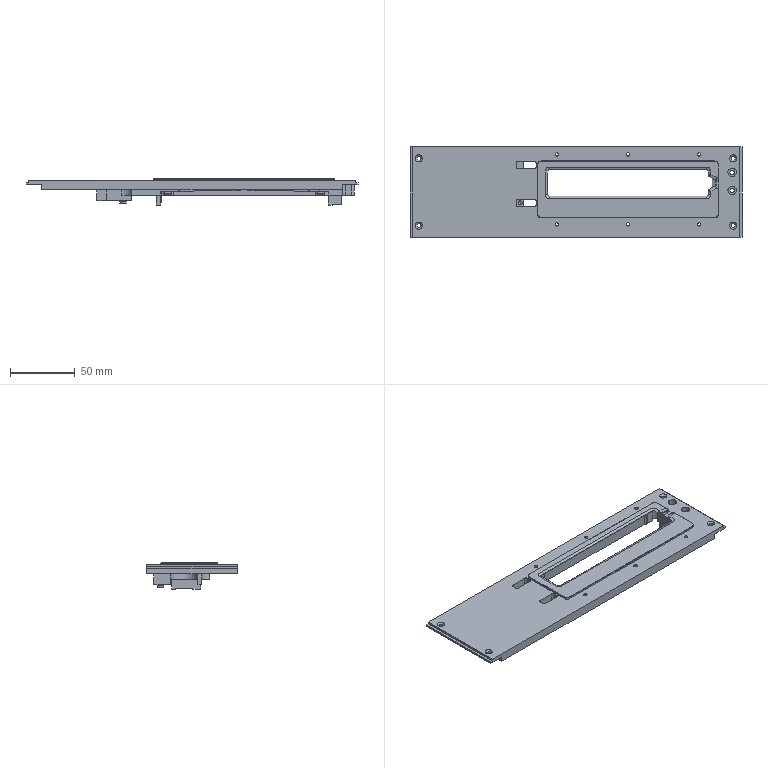NC program | NX | posted with a generic post | part box 256.6 x 70.3 x 20.422 mm
Lines 61 to 1223 of 23702:
(CAVITY_MILL , TOOL : D10)
N120 T10 M6
N122 G54
N124 G17 G0 G90 X-34.437 Y-41.146 S9500 M3
N126 G43 Z30. H10
N128 Z0.863
N130 G94 G1 Z-0.637 F1000.
N132 X-37.323 Y-36.146
N134 G3 X-38.189 Y-35.646 R1.
N136 G1 X-128.303 F3000.
N138 G2 X-128.797 Y-35.152 R0.494
N140 G1 Y35.152
N142 G2 X-128.303 Y35.646 R0.494
N144 G1 X128.303
N146 G2 X128.797 Y35.152 R0.494
N148 G1 Y-35.152
N150 G2 X128.303 Y-35.646 R0.494
N152 G1 X-38.189
N154 Y-29.646
N156 X-122.797
N158 Y29.646
N160 X122.797
N162 Y-29.646
N164 X-38.189
N166 Y-23.646
N168 X-116.797
N170 Y23.646
N172 X116.797
N174 Y-23.646
N176 X-38.189
N178 Y-17.646
N180 X-110.797
N182 Y-12.457
N184 G3 X-108.238 Y-13. R6.3
N186 G1 X-105.19
N188 G3 X-98.89 Y-6.7 R6.3
N190 G1 Y-0.604
N192 G3 X-105.19 Y5.696 R6.3
N194 G1 X-108.238
N196 G3 X-110.797 Y5.153 R6.3
N198 G1 X-110.31 Y4.056
N200 G2 X-108.238 Y4.496 R5.1
N202 G1 X-105.19
N204 G2 X-100.09 Y-0.604 R5.1
N206 G1 Y-6.7
N208 G2 X-105.19 Y-11.8 R5.1
N210 G1 X-108.238
N212 G2 X-113.338 Y-6.7 R5.1
N214 G1 Y-0.604
N216 G2 X-110.31 Y4.056 R5.1
N218 G1 X-110.797 Y5.153
N220 Y17.646
N222 X18.206
N224 G3 X17.898 Y15.7 R6.3
N226 G1 Y12.604
N228 G3 X24.198 Y6.304 R6.3
N230 G1 X27.754
N232 G3 X34.054 Y12.604 R6.3
N234 G1 Y15.7
N236 G3 X33.746 Y17.646 R6.3
N238 G1 X32.604 Y17.276
N240 G2 X32.854 Y15.7 R5.1
N242 G1 Y12.604
N244 G2 X27.754 Y7.504 R5.1
N246 G1 X24.198
N248 G2 X19.098 Y12.604 R5.1
N250 G1 Y15.7
N252 G2 X24.198 Y20.8 R5.1
N254 G1 X27.754
N256 G2 X32.604 Y17.276 R5.1
N258 G1 X33.746 Y17.646
N260 X110.797
N262 Y-17.646
N264 X31.656
N266 Y-11.646
N268 G3 X34.054 Y-6.7 R6.3
N270 G1 Y-0.604
N272 G3 X33.587 Y1.775 R6.3
N274 X40.016 Y11.646 R12.3
N276 G1 X104.797
N278 Y-11.646
N280 X31.656
N282 X40.054 Y-5.646
N284 Y-0.946
N286 G3 X44.68 Y5.646 R18.3
N288 G1 X98.797
N290 Y-5.646
N292 X40.054
N294 X45.941 Y-1.146
N296 G3 X47.466 Y1.146 R22.8
N298 G1 X94.297
N300 Y-1.146
N302 X45.941
N304 X40.054 Y-5.646
N306 X31.656 Y-11.646
N308 Y-17.646
N310 X-38.189
N312 Y-11.646
N314 X-93.928
N316 G3 X-92.89 Y-6.7 R12.3
N318 G1 Y-0.604
N320 G3 X-104.086 Y11.646 R12.3
N322 G1 X11.935
N324 G3 X18.364 Y1.775 R12.3
N326 X17.898 Y-0.604 R6.3
N328 G1 Y-6.7
N330 G3 X20.296 Y-11.646 R6.3
N332 G1 X21.039 Y-10.704
N334 G2 X19.098 Y-6.7 R5.1
N336 G1 Y-0.604
N338 G2 X24.198 Y4.496 R5.1
N340 G1 X27.754
N342 G2 X32.854 Y-0.604 R5.1
N344 G1 Y-6.7
N346 G2 X27.754 Y-11.8 R5.1
N348 G1 X24.198
N350 G2 X21.039 Y-10.704 R5.1
N352 G1 X20.296 Y-11.646
N354 X-38.189
N356 Y-5.646
N358 X-86.89
N360 Y-0.604
N362 G3 X-87.99 Y5.646 R18.3
N364 G1 X7.272
N366 G3 X11.898 Y-0.946 R18.3
N368 G1 Y-5.646
N370 X-38.189
N372 Y-1.146
N374 X-82.39
N376 Y-0.604
N378 G3 X-82.457 Y1.146 R22.8
N380 G1 X4.486
N382 G3 X6.011 Y-1.146 R22.8
N384 G1 X-38.189
N386 G3 X-39.056 Y-1.646 R1.
N388 G1 Z0.863
N390 G0 Z30.
N392 X-33.743 Y-41.146
N394 Z0.482
N396 G1 Z-1.018 F1000.
N398 X-36.63 Y-36.146
N400 G3 X-37.496 Y-35.646 R1.
N402 G1 X-128.303 F3000.
N404 G2 X-128.797 Y-35.152 R0.494
N406 G1 Y35.152
N408 G2 X-128.303 Y35.646 R0.494
N410 G1 X128.303
N412 G2 X128.797 Y35.152 R0.494
N414 G1 Y-35.152
N416 G2 X128.303 Y-35.646 R0.494
N418 G1 X-37.496
N420 Y-29.646
N422 X-122.797
N424 Y29.646
N426 X122.797
N428 Y-29.646
N430 X-37.496
N432 Y-23.646
N434 X-116.797
N436 Y-12.864
N438 G3 X-115.496 Y-13. R6.3
N440 G1 X-105.19
N442 G3 X-98.89 Y-6.7 R6.3
N444 G1 Y14.085
N446 G3 X-105.19 Y20.385 R6.3
N448 G1 X-115.496
N450 G3 X-116.797 Y20.249 R6.3
N452 G1 X-116.549 Y19.075
N454 G2 X-115.496 Y19.185 R5.1
N456 G1 X-105.19
N458 G2 X-100.09 Y14.085 R5.1
N460 G1 Y-6.7
N462 G2 X-105.19 Y-11.8 R5.1
N464 G1 X-115.496
N466 G2 X-120.596 Y-6.7 R5.1
N468 G1 Y14.085
N470 G2 X-116.549 Y19.075 R5.1
N472 G1 X-116.797 Y20.249
N474 Y23.646
N476 X116.797
N478 Y-23.646
N480 X-37.496
N482 Y-17.646
N484 X-99.58
N486 X-108.161 Y-18.324
N488 X-99.58 Y-17.646
N490 G3 X-92.89 Y-6.7 R12.3
N492 G1 Y14.085
N494 G3 X-93.417 Y17.646 R12.3
N496 G1 X18.206
N498 G3 X17.898 Y15.7 R6.3
N500 G1 Y12.604
N502 G3 X18.677 Y9.57 R6.3
N504 G1 Y2.43
N506 G3 X17.898 Y-0.604 R6.3
N508 G1 Y-6.7
N510 G3 X24.198 Y-13. R6.3
N512 G1 X27.754
N514 G3 X34.054 Y-6.7 R6.3
N516 G1 Y15.7
N518 G3 X33.746 Y17.646 R6.3
N520 G1 X32.604 Y17.276
N522 G2 X32.854 Y15.7 R5.1
N524 G1 Y-6.7
N526 G2 X27.754 Y-11.8 R5.1
N528 G1 X24.198
N530 G2 X19.098 Y-6.7 R5.1
N532 G1 Y-0.604
N534 G2 X19.877 Y2.105 R5.1
N536 G1 Y9.895
N538 G2 X19.098 Y12.604 R5.1
N540 G1 Y15.7
N542 G2 X24.198 Y20.8 R5.1
N544 G1 X27.754
N546 G2 X32.604 Y17.276 R5.1
N548 G1 X33.746 Y17.646
N550 X110.797
N552 Y-17.646
N554 X39.015
N556 Y-11.646
N558 G3 X40.054 Y-6.7 R12.3
N560 G1 Y11.646
N562 X104.797
N564 Y-11.646
N566 X39.015
N568 X46.054 Y-5.646
N570 Y5.646
N572 X98.797
N574 Y-5.646
N576 X46.054
N578 X50.554 Y-1.146
N580 Y1.146
N582 X94.297
N584 Y-1.146
N586 X50.554
N588 X46.054 Y-5.646
N590 X39.015 Y-11.646
N592 Y-17.646
N594 X-37.496
N596 Y-11.646
N598 X-87.571
N600 G3 X-86.89 Y-6.7 R18.3
N602 G1 Y11.646
N604 X11.935
N606 G3 X12.677 Y8.297 R12.3
N608 G1 Y3.703
N610 G3 X11.898 Y-0.604 R12.3
N612 G1 Y-6.7
N614 G3 X12.936 Y-11.646 R12.3
N616 G1 X-37.496
N618 Y-5.646
N620 X-80.89
N622 Y5.646
N624 X6.677
N626 Y4.677
N628 G3 X5.898 Y-0.604 R18.3
N630 G1 Y-5.646
N632 X-37.496
N634 Y-1.146
N636 X-76.39
N638 Y1.146
N640 X1.465
N642 G3 X1.398 Y-0.604 R22.8
N644 G1 Y-1.146
N646 X-37.496
N648 G3 X-38.362 Y-1.646 R1.
N650 G1 Z0.482
N652 G0 Z30.
N654 X-33.743 Y-41.146
N656 Z0.078
N658 G1 Z-1.422 F1000.
N660 X-36.63 Y-36.146
N662 G3 X-37.496 Y-35.646 R1.
N664 G1 X-128.303 F3000.
N666 G2 X-128.797 Y-35.152 R0.495
N668 G1 Y35.152
N670 G2 X-128.303 Y35.646 R0.495
N672 G1 X128.303
N674 G2 X128.797 Y35.152 R0.495
N676 G1 Y-35.152
N678 G2 X128.303 Y-35.646 R0.495
N680 G1 X-37.496
N682 Y-29.646
N684 X-122.797
N686 Y29.646
N688 X122.797
N690 Y-29.646
N692 X-37.496
N694 Y-23.646
N696 X-116.797
N698 Y-12.864
N700 G3 X-115.496 Y-13. R6.3
N702 G1 X-105.19
N704 G3 X-98.89 Y-6.7 R6.3
N706 G1 Y14.085
N708 G3 X-105.19 Y20.385 R6.3
N710 G1 X-115.496
N712 G3 X-116.797 Y20.249 R6.3
N714 G1 X-116.549 Y19.075
N716 G2 X-115.496 Y19.185 R5.1
N718 G1 X-105.19
N720 G2 X-100.09 Y14.085 R5.1
N722 G1 Y-6.7
N724 G2 X-105.19 Y-11.8 R5.1
N726 G1 X-115.496
N728 G2 X-120.596 Y-6.7 R5.1
N730 G1 Y14.085
N732 G2 X-116.549 Y19.075 R5.1
N734 G1 X-116.797 Y20.249
N736 Y23.646
N738 X116.797
N740 Y-23.646
N742 X-37.496
N744 Y-17.646
N746 X-99.58
N748 X-108.161 Y-18.324
N750 X-99.58 Y-17.646
N752 G3 X-92.89 Y-6.7 R12.3
N754 G1 Y14.085
N756 G3 X-93.417 Y17.646 R12.3
N758 G1 X18.206
N760 G3 X17.898 Y15.7 R6.3
N762 G1 Y12.604
N764 G3 X18.273 Y10.464 R6.3
N766 G1 Y1.536
N768 G3 X17.898 Y-0.604 R6.3
N770 G1 Y-6.7
N772 G3 X24.198 Y-13. R6.3
N774 G1 X27.754
N776 G3 X34.054 Y-6.7 R6.3
N778 G1 Y15.7
N780 G3 X33.746 Y17.646 R6.3
N782 G1 X32.604 Y17.276
N784 G2 X32.854 Y15.7 R5.1
N786 G1 Y-6.7
N788 G2 X27.754 Y-11.8 R5.1
N790 G1 X24.198
N792 G2 X19.098 Y-6.7 R5.1
N794 G1 Y-0.604
N796 G2 X19.473 Y1.315 R5.1
N798 G1 Y10.685
N800 G2 X19.098 Y12.604 R5.1
N802 G1 Y15.7
N804 G2 X24.198 Y20.8 R5.1
N806 G1 X27.754
N808 G2 X32.604 Y17.276 R5.1
N810 G1 X33.746 Y17.646
N812 X110.797
N814 Y-17.646
N816 X39.015
N818 Y-11.646
N820 G3 X40.054 Y-6.7 R12.3
N822 G1 Y11.646
N824 X104.797
N826 Y-11.646
N828 X39.015
N830 X46.054 Y-5.646
N832 Y5.646
N834 X98.797
N836 Y-5.646
N838 X46.054
N840 X50.554 Y-1.146
N842 Y1.146
N844 X94.297
N846 Y-1.146
N848 X50.554
N850 X46.054 Y-5.646
N852 X39.015 Y-11.646
N854 Y-17.646
N856 X-37.496
N858 Y-11.646
N860 X-87.571
N862 G3 X-86.89 Y-6.7 R18.3
N864 G1 Y11.646
N866 X11.935
N868 G3 X12.273 Y9.591 R12.3
N870 G1 Y2.409
N872 G3 X11.898 Y-0.604 R12.3
N874 G1 Y-6.7
N876 G3 X12.936 Y-11.646 R12.3
N878 G1 X-37.496
N880 Y-5.646
N882 X-80.89
N884 Y5.646
N886 X6.273
N888 Y3.08
N890 G3 X5.898 Y-0.604 R18.3
N892 G1 Y-5.646
N894 X-37.496
N896 Y-1.146
N898 X-76.39
N900 Y1.146
N902 X1.465
N904 G3 X1.398 Y-0.604 R22.8
N906 G1 Y-1.146
N908 X-37.496
N910 G3 X-38.362 Y-1.646 R1.
N912 G1 Z0.078
N914 G0 X-33.743 Y-41.147 Z-0.922
N916 G1 Z-2.422 F1000.
N918 X-36.63 Y-36.147
N920 G3 X-37.496 Y-35.647 R1.
N922 G1 X-128.302 F3000.
N924 G2 X-128.797 Y-35.152 R0.495
N926 G1 Y35.152
N928 G2 X-128.302 Y35.647 R0.495
N930 G1 X128.302
N932 G2 X128.797 Y35.152 R0.495
N934 G1 Y-35.152
N936 G2 X128.302 Y-35.647 R0.495
N938 G1 X-37.496
N940 Y-29.647
N942 X-122.797
N944 Y29.647
N946 X46.173
N948 G3 X60.355 Y29.647 R-8.792
N950 G1 X59.387 Y28.937
N952 G2 X57.751 Y18.327 R7.592
N954 X59.387 Y28.937 R-7.592
N956 G1 X60.355 Y29.647
N958 X122.797
N960 Y-29.647
N962 X-37.496
N964 Y-23.647
N966 X-116.797
N968 Y-12.864
N970 G3 X-115.496 Y-13. R6.3
N972 G1 X-105.19
N974 G3 X-98.89 Y-6.7 R6.3
N976 G1 Y14.085
N978 G3 X-105.19 Y20.385 R6.3
N980 G1 X-115.496
N982 G3 X-116.797 Y20.249 R6.3
N984 G1 X-116.549 Y19.075
N986 G2 X-115.496 Y19.185 R5.1
N988 G1 X-105.19
N990 G2 X-100.09 Y14.085 R5.1
N992 G1 Y-6.7
N994 G2 X-105.19 Y-11.8 R5.1
N996 G1 X-115.496
N998 G2 X-120.596 Y-6.7 R5.1
N1000 G1 Y14.085
N1002 G2 X-116.549 Y19.075 R5.1
N1004 G1 X-116.797 Y20.249
N1006 Y23.647
N1008 X38.494
N1010 G3 X68.034 Y23.647 R14.792
N1012 G1 X116.797
N1014 Y-23.647
N1016 X-37.496
N1018 Y-17.647
N1020 X-99.581
N1022 X-108.162 Y-18.324
N1024 X-99.581 Y-17.647
N1026 G3 X-92.89 Y-6.7 R12.3
N1028 G1 Y14.085
N1030 G3 X-93.417 Y17.647 R12.3
N1032 G1 X18.206
N1034 G3 X17.898 Y15.7 R6.3
N1036 G1 Y10.868
N1038 G3 X17.491 Y8.642 R6.3
N1040 G1 Y3.358
N1042 G3 X17.898 Y1.132 R6.3
N1044 G1 Y-6.7
N1046 G3 X24.198 Y-13. R6.3
N1048 G1 X27.754
N1050 G3 X34.054 Y-6.7 R6.3
N1052 G1 Y15.7
N1054 G3 X33.976 Y16.687 R6.3
N1056 G1 X32.791 Y16.499
N1058 G2 X32.854 Y15.7 R5.1
N1060 G1 Y-6.7
N1062 G2 X27.754 Y-11.8 R5.1
N1064 G1 X24.198
N1066 G2 X19.098 Y-6.7 R5.1
N1068 G1 Y1.363
N1070 G2 X18.691 Y3.358 R5.1
N1072 G1 Y8.642
N1074 G2 X19.098 Y10.637 R5.1
N1076 G1 Y15.7
N1078 G2 X24.198 Y20.8 R5.1
N1080 G1 X27.754
N1082 G2 X32.791 Y16.499 R5.1
N1084 G1 X33.976 Y16.687
N1086 G3 X72.911 Y17.647 R20.792
N1088 G1 X110.797
N1090 Y-17.647
N1092 X39.015
N1094 Y-11.647
N1096 G3 X40.054 Y-6.647 R12.3
N1098 G1 X45.576 Y-6.521
N1100 X40.054 Y-6.647
N1102 Y1.142
N1104 G3 X76.798 Y11.647 R26.792
N1106 G1 X104.797
N1108 Y-11.647
N1110 X66.283
N1112 Y-5.647
N1114 G3 X80.129 Y5.647 R32.792
N1116 G1 X98.797
N1118 Y-5.647
N1120 X80.384
N1122 Y-1.147
N1124 G3 X82.378 Y1.147 R37.292
N1126 G1 X94.297
N1128 Y-1.147
N1130 X80.384
N1132 Y-5.647
N1134 X66.283
N1136 X60.869 Y-6.534
N1138 X66.283 Y-5.647
N1140 Y-11.647
N1142 X39.015
N1144 Y-17.647
N1146 X-37.496
N1148 Y-11.647
N1150 X-87.571
N1152 G3 X-86.89 Y-6.7 R18.3
N1154 G1 Y11.647
N1156 X11.864
N1158 G3 X11.491 Y8.642 R12.3
N1160 G1 Y3.358
N1162 G3 X11.898 Y0.223 R12.3
N1164 G1 Y-6.7
N1166 G3 X12.936 Y-11.647 R12.3
N1168 G1 X-37.496
N1170 Y-5.647
N1172 X-80.89
N1174 Y5.647
N1176 X5.491
N1178 Y3.358
N1180 G3 X5.898 Y-0.477 R18.3
N1182 G1 Y-5.647
N1184 X-37.496
N1186 Y-1.147
N1188 X-76.39
N1190 Y1.147
N1192 X1.099
N1194 G3 X1.398 Y-0.927 R22.8
N1196 G1 Y-1.147
N1198 X-37.496
N1200 G3 X-38.362 Y-1.647 R1.
N1202 G1 Z-0.922
N1204 G0 X-33.743 Y-41.147 Z-1.922
N1206 G1 Z-3.422 F1000.
N1208 X-36.63 Y-36.147
N1210 G3 X-37.496 Y-35.647 R1.
N1212 G1 X-128.302 F3000.
N1214 G2 X-128.797 Y-35.152 R0.495
N1216 G1 Y35.152
N1218 G2 X-128.302 Y35.647 R0.495
N1220 G1 X128.302
N1222 G2 X128.797 Y35.152 R0.495
N1224 G1 Y-35.152
N1226 G2 X128.302 Y-35.647 R0.495
N1228 G1 X-37.496
N1230 Y-29.647
N1232 X-122.797
N1234 Y29.647
N1236 X46.162
N1238 G3 X60.366 Y29.647 R-8.8
N1240 G1 X59.397 Y28.938
N1242 G2 X57.752 Y18.317 R7.6
N1244 X59.397 Y28.938 R-7.6
N1246 G1 X60.366 Y29.647
N1248 X122.797
N1250 Y-29.647
N1252 X-37.496
N1254 Y-23.647
N1256 X-116.797
N1258 Y-12.864
N1260 G3 X-115.496 Y-13. R6.3
N1262 G1 X-105.19
N1264 G3 X-98.89 Y-6.7 R6.3
N1266 G1 Y14.085
N1268 G3 X-105.19 Y20.385 R6.3
N1270 G1 X-115.496
N1272 G3 X-116.797 Y20.249 R6.3
N1274 G1 X-116.55 Y19.075
N1276 G2 X-115.496 Y19.185 R5.1
N1278 G1 X-105.19
N1280 G2 X-100.09 Y14.085 R5.1
N1282 G1 Y-6.7
N1284 G2 X-105.19 Y-11.8 R5.1
N1286 G1 X-115.496
N1288 G2 X-120.596 Y-6.7 R5.1
N1290 G1 Y14.085
N1292 G2 X-116.55 Y19.075 R5.1
N1294 G1 X-116.797 Y20.249
N1296 Y23.647
N1298 X38.486
N1300 G3 X68.042 Y23.647 R14.8
N1302 G1 X116.797
N1304 Y-23.647
N1306 X-37.496
N1308 Y-17.647
N1310 X-99.581
N1312 X-108.162 Y-18.324
N1314 X-99.581 Y-17.647
N1316 G3 X-92.89 Y-6.7 R12.3
N1318 G1 Y14.085
N1320 G3 X-93.417 Y17.647 R12.3
N1322 G1 X18.206
N1324 G3 X17.898 Y15.7 R6.3
N1326 G1 Y10.868
N1328 G3 X17.491 Y8.642 R6.3
N1330 G1 Y3.358
N1332 G3 X17.898 Y1.132 R6.3
N1334 G1 Y-6.7
N1336 G3 X24.198 Y-13. R6.3
N1338 G1 X27.754
N1340 G3 X34.054 Y-6.7 R6.3
N1342 G1 Y15.7
N1344 G3 X33.982 Y16.65 R6.3
N1346 G1 X32.795 Y16.469
N1348 G2 X32.854 Y15.7 R5.1
N1350 G1 Y-6.7
N1352 G2 X27.754 Y-11.8 R5.1
N1354 G1 X24.198
N1356 G2 X19.098 Y-6.7 R5.1
N1358 G1 Y1.363
N1360 G2 X18.691 Y3.358 R5.1
N1362 G1 Y8.642
N1364 G2 X19.098 Y10.637 R5.1
N1366 G1 Y15.7
N1368 G2 X24.198 Y20.8 R5.1
N1370 G1 X27.754
N1372 G2 X32.795 Y16.469 R5.1
N1374 G1 X33.982 Y16.65
N1376 G3 X72.92 Y17.647 R20.8
N1378 G1 X110.797
N1380 Y-17.647
N1382 X39.015
N1384 Y-11.647
N1386 G3 X40.054 Y-6.647 R12.3
N1388 G1 X45.564 Y-6.524
N1390 X40.054 Y-6.647
N1392 Y1.132
N1394 G3 X76.808 Y11.647 R26.8
N1396 G1 X104.797
N1398 Y-11.647
N1400 X66.303
N1402 Y-5.647
N1404 G3 X80.139 Y5.647 R32.8
N1406 G1 X98.797
N1408 Y-5.647
N1410 X80.395
N1412 Y-1.147
N1414 G3 X82.389 Y1.147 R37.3
N1416 G1 X94.297
N1418 Y-1.147
N1420 X80.395
N1422 Y-5.647
N1424 X66.303
N1426 X60.896 Y-6.535
N1428 X66.303 Y-5.647
N1430 Y-11.647
N1432 X39.015
N1434 Y-17.647
N1436 X-37.496
N1438 Y-11.647
N1440 X-87.571
N1442 G3 X-86.89 Y-6.7 R18.3
N1444 G1 Y11.647
N1446 X11.864
N1448 G3 X11.491 Y8.642 R12.3
N1450 G1 Y3.358
N1452 G3 X11.898 Y0.223 R12.3
N1454 G1 Y-6.7
N1456 G3 X12.936 Y-11.647 R12.3
N1458 G1 X-37.496
N1460 Y-5.647
N1462 X-80.89
N1464 Y5.647
N1466 X5.491
N1468 Y3.358
N1470 G3 X5.898 Y-0.477 R18.3
N1472 G1 Y-5.647
N1474 X-37.496
N1476 Y-1.147
N1478 X-76.39
N1480 Y1.147
N1482 X1.099
N1484 G3 X1.398 Y-0.927 R22.8
N1486 G1 Y-1.147
N1488 X-37.496
N1490 G3 X-38.362 Y-1.647 R1.
N1492 G1 Z-1.922
N1494 G0 X-33.743 Y-41.147 Z-2.762
N1496 G1 Z-4.262 F1000.
N1498 X-36.63 Y-36.147
N1500 G3 X-37.496 Y-35.647 R1.
N1502 G1 X-128.302 F3000.
N1504 G2 X-128.798 Y-35.152 R0.495
N1506 G1 Y35.152
N1508 G2 X-128.302 Y35.647 R0.495
N1510 G1 X45.124
N1512 G2 X46.504 Y35.8 R6.3
N1514 G1 X73.504
N1516 G2 X74.884 Y35.647 R6.3
N1518 G1 X128.302
N1520 G2 X128.798 Y35.152 R0.495
N1522 G1 Y-35.152
N1524 G2 X128.302 Y-35.647 R0.495
N1526 G1 X-37.496
N1528 Y-29.647
N1530 X-122.798
N1532 Y29.647
N1534 X40.206
N1536 X40.204 Y29.5
N1538 Y17.029
N1540 Y16.501
N1542 G3 X46.504 Y10.2 R6.301
N1544 G1 X73.504
N1546 G3 X79.804 Y16.5 R6.3
N1548 G1 Y29.5
N1550 X79.802 Y29.647
N1552 X78.603 Y29.619
N1554 X78.604 Y29.5
N1556 Y16.5
N1558 G2 X73.504 Y11.4 R5.1
N1560 G1 X46.504
N1562 G2 X41.404 Y16.5 R5.101
N1564 G1 Y17.029
N1566 Y29.5
N1568 G2 X46.504 Y34.6 R5.1
N1570 G1 X73.504
N1572 G2 X78.603 Y29.619 R5.1
N1574 G1 X79.802 Y29.647
N1576 X122.798
N1578 Y-29.647
N1580 X-37.496
N1582 Y-23.647
N1584 X-116.798
N1586 Y-12.864
N1588 G3 X-115.496 Y-13. R6.3
N1590 G1 X-105.19
N1592 G3 X-98.89 Y-6.7 R6.3
N1594 G1 Y14.085
N1596 G3 X-105.19 Y20.385 R6.3
N1598 G1 X-115.496
N1600 G3 X-116.798 Y20.249 R6.3
N1602 G1 X-116.55 Y19.075
N1604 G2 X-115.496 Y19.185 R5.1
N1606 G1 X-105.19
N1608 G2 X-100.09 Y14.085 R5.1
N1610 G1 Y-6.7
N1612 G2 X-105.19 Y-11.8 R5.1
N1614 G1 X-115.496
N1616 G2 X-120.596 Y-6.7 R5.1
N1618 G1 Y14.085
N1620 G2 X-116.55 Y19.075 R5.1
N1622 G1 X-116.798 Y20.249
N1624 Y23.647
N1626 X34.204
N1628 Y17.031
N1630 Y16.5
N1632 G3 X46.502 Y4.2 R12.301
N1634 G1 X73.504
N1636 G3 X85.804 Y16.5 R12.3
N1638 G1 Y23.647
N1640 X116.798
N1642 Y-23.647
N1644 X-37.496
N1646 Y-17.647
N1648 X-99.581
N1650 X-108.162 Y-18.324
N1652 X-99.581 Y-17.647
N1654 G3 X-92.89 Y-6.7 R12.3
N1656 G1 Y14.085
N1658 G3 X-93.417 Y17.647 R12.3
N1660 G1 X18.206
N1662 G3 X17.898 Y15.7 R6.3
N1664 G1 Y10.868
N1666 G3 X17.491 Y8.642 R6.3
N1668 G1 Y3.358
N1670 G3 X17.898 Y1.132 R6.3
N1672 G1 Y-6.7
N1674 G3 X24.198 Y-13. R6.3
N1676 G1 X27.754
N1678 G3 X34.054 Y-6.7 R6.3
N1680 G1 Y3.088
N1682 X32.854
N1684 Y-6.7
N1686 G2 X27.754 Y-11.8 R5.1
N1688 G1 X24.198
N1690 G2 X19.098 Y-6.7 R5.1
N1692 G1 Y1.363
N1694 G2 X18.691 Y3.358 R5.1
N1696 G1 Y8.642
N1698 G2 X19.098 Y10.637 R5.1
N1700 G1 Y15.7
N1702 G2 X24.198 Y20.8 R5.1
N1704 G1 X27.754
N1706 G2 X32.854 Y15.7 R5.1
N1708 G1 Y3.088
N1710 X34.054
N1712 G3 X41.247 Y-1.028 R18.301
N1714 X40.204 Y-4.5 R6.3
N1716 G1 Y-7.5
N1718 G3 X46.504 Y-13.8 R6.3
N1720 G1 X66.004
N1722 G3 X72.304 Y-7.5 R6.3
N1724 G1 Y-4.5
N1726 G3 X71.696 Y-1.8 R6.3
N1728 G1 X70.612 Y-2.314
N1730 G2 X71.104 Y-4.5 R5.1
N1732 G1 Y-7.5
N1734 G2 X66.004 Y-12.6 R5.1
N1736 G1 X46.504
N1738 G2 X41.404 Y-7.5 R5.1
N1740 G1 Y-4.5
N1742 G2 X46.504 Y0.6 R5.1
N1744 G1 X66.004
N1746 G2 X70.612 Y-2.314 R5.1
N1748 G1 X71.696 Y-1.8
N1750 X73.504
N1752 G3 X91.804 Y16.5 R18.3
N1754 G1 Y17.647
N1756 X110.798
N1758 Y-17.647
N1760 X77.584
N1762 Y-11.647
N1764 G3 X78.304 Y-7.5 R12.3
N1766 G1 Y-7.321
N1768 G3 X97.314 Y11.647 R24.3
N1770 G1 X104.798
N1772 Y-11.647
N1774 X94.183
N1776 Y-5.647
N1778 G3 X98.798 Y-0.183 R30.3
N1780 G1 Y-5.647
N1782 X94.183
N1784 Y-11.647
N1786 X77.584
N1788 Y-17.647
N1790 X-37.496
N1792 Y-11.647
N1794 X-87.571
N1796 G3 X-86.89 Y-6.7 R18.3
N1798 G1 Y11.647
N1800 X11.864
N1802 G3 X11.491 Y8.642 R12.3
N1804 G1 Y3.358
N1806 G3 X11.898 Y0.223 R12.3
N1808 G1 Y-6.7
N1810 G3 X12.937 Y-11.647 R12.3
N1812 G1 X-37.496
N1814 Y-5.647
N1816 X-80.89
N1818 Y5.647
N1820 X5.491
N1822 Y3.358
N1824 G3 X5.898 Y-0.477 R18.3
N1826 G1 Y-5.647
N1828 X-37.496
N1830 Y-1.147
N1832 X-76.39
N1834 Y1.147
N1836 X1.099
N1838 G3 X1.398 Y-0.927 R22.8
N1840 G1 Y-1.147
N1842 X-37.496
N1844 G3 X-38.362 Y-1.647 R1.
N1846 G1 Z-2.762
N1848 G0 X-33.743 Y-41.147 Z-3.602
N1850 G1 Z-5.102 F1000.
N1852 X-36.63 Y-36.147
N1854 G3 X-37.496 Y-35.647 R1.
N1856 G1 X-128.302 F3000.
N1858 G2 X-128.798 Y-35.152 R0.496
N1860 G1 Y35.152
N1862 G2 X-128.302 Y35.647 R0.496
N1864 G1 X45.125
N1866 G2 X46.504 Y35.8 R6.3
N1868 G1 X73.504
N1870 G2 X74.883 Y35.647 R6.3
N1872 G1 X128.302
N1874 G2 X128.798 Y35.152 R0.496
N1876 G1 Y-35.152
N1878 G2 X128.302 Y-35.647 R0.496
N1880 G1 X-37.496
N1882 Y-29.647
N1884 X-122.798
N1886 Y29.647
N1888 X40.206
N1890 X40.204 Y29.5
N1892 Y23.647
N1894 Y17.02
N1896 X40.209 Y16.431
N1898 G3 X46.488 Y10.2 R6.28
N1900 G1 X73.504
N1902 G3 X79.804 Y16.5 R6.3
N1904 G1 Y29.5
N1906 X79.802 Y29.647
N1908 X78.603 Y29.619
N1910 X78.604 Y29.5
N1912 Y16.5
N1914 G2 X73.504 Y11.4 R5.1
N1916 G1 X46.488
N1918 G2 X41.409 Y16.441 R5.08
N1920 G1 X41.404 Y17.029
N1922 Y29.5
N1924 G2 X46.504 Y34.6 R5.1
N1926 G1 X73.504
N1928 G2 X78.603 Y29.619 R5.1
N1930 G1 X79.802 Y29.647
N1932 X122.798
N1934 Y-29.647
N1936 X-37.496
N1938 Y-23.647
N1940 X-116.798
N1942 Y-12.864
N1944 G3 X-115.496 Y-13. R6.3
N1946 G1 X-105.19
N1948 G3 X-98.89 Y-6.7 R6.3
N1950 G1 Y14.085
N1952 G3 X-105.19 Y20.385 R6.3
N1954 G1 X-115.496
N1956 G3 X-116.798 Y20.249 R6.3
N1958 G1 X-116.55 Y19.075
N1960 G2 X-115.496 Y19.185 R5.1
N1962 G1 X-105.19
N1964 G2 X-100.09 Y14.085 R5.1
N1966 G1 Y-6.7
N1968 G2 X-105.19 Y-11.8 R5.1
N1970 G1 X-115.496
N1972 G2 X-120.596 Y-6.7 R5.1
N1974 G1 Y14.085
N1976 G2 X-116.55 Y19.075 R5.1
N1978 G1 X-116.798 Y20.249
N1980 Y23.647
N1982 X34.204
N1984 Y16.985
N1986 X34.209 Y16.385
N1988 G3 X46.488 Y4.2 R12.28
N1990 G1 X73.504
N1992 G3 X85.804 Y16.5 R12.3
N1994 G1 Y23.647
N1996 X116.798
N1998 Y-23.647
N2000 X-37.496
N2002 Y-17.647
N2004 X-99.582
N2006 X-108.162 Y-18.324
N2008 X-99.582 Y-17.647
N2010 G3 X-92.89 Y-6.7 R12.3
N2012 G1 Y14.085
N2014 G3 X-93.417 Y17.647 R12.3
N2016 G1 X18.206
N2018 G3 X17.898 Y15.7 R6.3
N2020 G1 Y10.868
N2022 G3 X17.491 Y8.642 R6.3
N2024 G1 Y3.358
N2026 G3 X17.898 Y1.132 R6.3
N2028 G1 Y-6.7
N2030 G3 X24.198 Y-13. R6.3
N2032 G1 X27.754
N2034 G3 X34.054 Y-6.7 R6.3
N2036 G1 Y3.081
N2038 X32.854
N2040 Y-6.7
N2042 G2 X27.754 Y-11.8 R5.1
N2044 G1 X24.198
N2046 G2 X19.098 Y-6.7 R5.1
N2048 G1 Y1.363
N2050 G2 X18.691 Y3.358 R5.1
N2052 G1 Y8.642
N2054 G2 X19.098 Y10.637 R5.1
N2056 G1 Y15.7
N2058 G2 X24.198 Y20.8 R5.1
N2060 G1 X27.754
N2062 G2 X32.854 Y15.7 R5.1
N2064 G1 Y3.081
N2066 X34.054
N2068 G3 X41.245 Y-1.032 R18.28
N2070 X40.204 Y-4.5 R6.3
N2072 G1 Y-7.5
N2074 G3 X46.504 Y-13.8 R6.3
N2076 G1 X66.004
N2078 G3 X72.304 Y-7.5 R6.3
N2080 G1 Y-4.5
N2082 G3 X71.696 Y-1.8 R6.3
N2084 G1 X70.612 Y-2.314
N2086 G2 X71.104 Y-4.5 R5.1
N2088 G1 Y-7.5
N2090 G2 X66.004 Y-12.6 R5.1
N2092 G1 X46.504
N2094 G2 X41.404 Y-7.5 R5.1
N2096 G1 Y-4.5
N2098 G2 X46.504 Y0.6 R5.1
N2100 G1 X66.004
N2102 G2 X70.612 Y-2.314 R5.1
N2104 G1 X71.696 Y-1.8
N2106 X73.504
N2108 G3 X91.804 Y16.5 R18.3
N2110 G1 Y17.647
N2112 X110.798
N2114 Y-17.647
N2116 X77.584
N2118 Y-11.647
N2120 G3 X78.304 Y-7.5 R12.3
N2122 G1 Y-7.321
N2124 G3 X97.315 Y11.647 R24.3
N2126 G1 X104.798
N2128 Y-11.647
N2130 X94.182
N2132 Y-5.647
N2134 G3 X98.798 Y-0.183 R30.3
N2136 G1 Y-5.647
N2138 X94.182
N2140 Y-11.647
N2142 X77.584
N2144 Y-17.647
N2146 X-37.496
N2148 Y-11.647
N2150 X-87.571
N2152 G3 X-86.89 Y-6.7 R18.3
N2154 G1 Y11.647
N2156 X11.864
N2158 G3 X11.491 Y8.642 R12.3
N2160 G1 Y3.358
N2162 G3 X11.898 Y0.223 R12.3
N2164 G1 Y-6.7
N2166 G3 X12.937 Y-11.647 R12.3
N2168 G1 X-37.496
N2170 Y-5.647
N2172 X-80.89
N2174 Y5.647
N2176 X5.491
N2178 Y3.358
N2180 G3 X5.898 Y-0.477 R18.3
N2182 G1 Y-5.647
N2184 X-37.496
N2186 Y-1.147
N2188 X-76.39
N2190 Y1.147
N2192 X1.099
N2194 G3 X1.398 Y-0.927 R22.8
N2196 G1 Y-1.147
N2198 X-37.496
N2200 G3 X-38.362 Y-1.647 R1.
N2202 G1 Z-3.602
N2204 G0 X-33.743 Y-41.147 Z-4.442
N2206 G1 Z-5.942 F1000.
N2208 X-36.63 Y-36.147
N2210 G3 X-37.496 Y-35.647 R1.
N2212 G1 X-128.302 F3000.
N2214 G2 X-128.798 Y-35.152 R0.496
N2216 G1 Y35.152
N2218 G2 X-128.302 Y35.647 R0.496
N2220 G1 X45.125
N2222 G2 X46.504 Y35.8 R6.3
N2224 G1 X73.504
N2226 G2 X74.883 Y35.647 R6.3
N2228 G1 X128.302
N2230 G2 X128.798 Y35.152 R0.496
N2232 G1 Y-35.152
N2234 G2 X128.302 Y-35.647 R0.496
N2236 G1 X-37.496
N2238 Y-29.647
N2240 X-122.798
N2242 Y29.647
N2244 X40.206
N2246 X40.204 Y29.5
N2248 Y23.647
N2250 Y17.02
N2252 X40.208 Y16.433
N2254 G3 X46.488 Y10.2 R6.28
N2256 G1 X73.504
N2258 G3 X79.804 Y16.5 R6.3
N2260 G1 Y29.5
N2262 X79.802 Y29.647
N2264 X78.603 Y29.619
N2266 X78.604 Y29.5
N2268 Y16.5
N2270 G2 X73.504 Y11.4 R5.1
N2272 G1 X46.488
N2274 G2 X41.408 Y16.442 R5.08
N2276 G1 X41.404 Y17.029
N2278 Y29.5
N2280 G2 X46.504 Y34.6 R5.1
N2282 G1 X73.504
N2284 G2 X78.603 Y29.619 R5.1
N2286 G1 X79.802 Y29.647
N2288 X122.798
N2290 Y-29.647
N2292 X-37.496
N2294 Y-23.647
N2296 X-116.798
N2298 Y-12.864
N2300 G3 X-115.496 Y-13. R6.3
N2302 G1 X-105.19
N2304 G3 X-98.89 Y-6.7 R6.3
N2306 G1 Y14.085
N2308 G3 X-105.19 Y20.385 R6.3
N2310 G1 X-115.496
N2312 G3 X-116.798 Y20.249 R6.3
N2314 G1 X-116.55 Y19.075
N2316 G2 X-115.496 Y19.185 R5.1
N2318 G1 X-105.19
N2320 G2 X-100.09 Y14.085 R5.1
N2322 G1 Y-6.7
N2324 G2 X-105.19 Y-11.8 R5.1
N2326 G1 X-115.496
N2328 G2 X-120.596 Y-6.7 R5.1
N2330 G1 Y14.085
N2332 G2 X-116.55 Y19.075 R5.1
N2334 G1 X-116.798 Y20.249
N2336 Y23.647
N2338 X34.204
N2340 Y16.986
N2342 X34.209 Y16.388
N2344 G3 X46.488 Y4.2 R12.28
N2346 G1 X73.504
N2348 G3 X85.804 Y16.5 R12.3
N2350 G1 Y23.647
N2352 X116.798
N2354 Y-23.647
N2356 X-37.496
N2358 Y-17.647
N2360 X-99.582
N2362 X-108.163 Y-18.324
N2364 X-99.582 Y-17.647
N2366 G3 X-92.89 Y-6.7 R12.3
N2368 G1 Y14.085
N2370 G3 X-93.417 Y17.647 R12.3
N2372 G1 X18.206
N2374 G3 X17.898 Y15.7 R6.3
N2376 G1 Y10.868
N2378 G3 X17.491 Y8.642 R6.3
N2380 G1 Y3.358
N2382 G3 X17.898 Y1.132 R6.3
N2384 G1 Y-6.7
N2386 G3 X24.198 Y-13. R6.3
N2388 G1 X27.754
N2390 G3 X34.054 Y-6.7 R6.3
N2392 G1 Y3.081
N2394 X32.854
N2396 Y-6.7
N2398 G2 X27.754 Y-11.8 R5.1
N2400 G1 X24.198
N2402 G2 X19.098 Y-6.7 R5.1
N2404 G1 Y1.363
N2406 G2 X18.691 Y3.358 R5.1
N2408 G1 Y8.642
N2410 G2 X19.098 Y10.637 R5.1
N2412 G1 Y15.7
N2414 G2 X24.198 Y20.8 R5.1
N2416 G1 X27.754
N2418 G2 X32.854 Y15.7 R5.1
N2420 G1 Y3.081
N2422 X34.054
N2424 G3 X41.245 Y-1.032 R18.28
N2426 X40.204 Y-4.5 R6.3
N2428 G1 Y-7.5
N2430 G3 X46.504 Y-13.8 R6.3
N2432 G1 X66.004
N2434 G3 X72.304 Y-7.5 R6.3
N2436 G1 Y-4.5
N2438 G3 X71.696 Y-1.8 R6.3